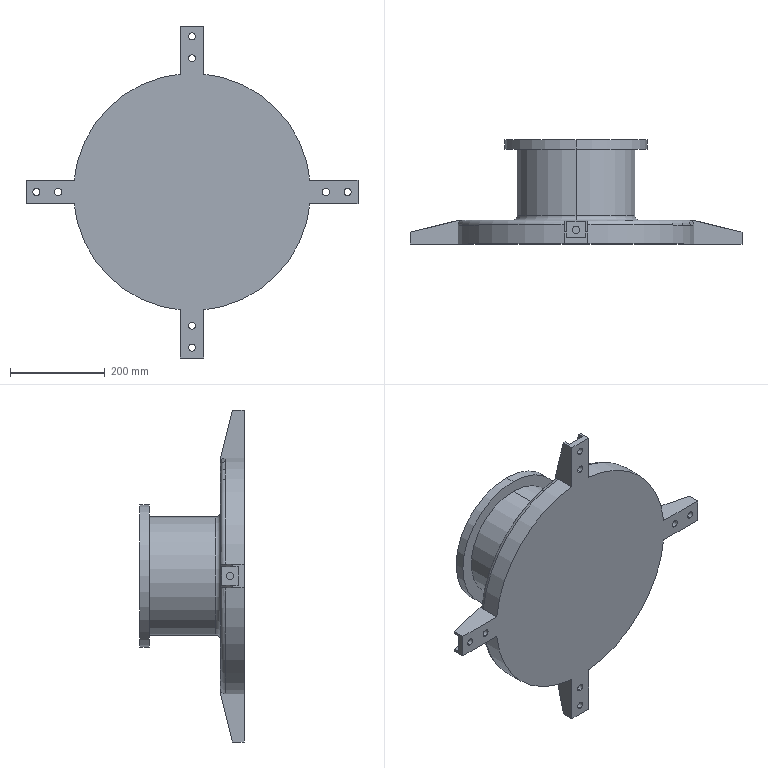Part | SolidWorks | features HoleWzd 6, ICE 5, BaseBody 1, Fillet 1, Revolution 1 | 1 solid | 81 faces | box 700 x 220 x 700 mm | volume 17727332 mm3 | plane 41 | cylinder 34 | torus 6 | commonest cylinder face diameters 15 x24 500 x4 125 x2 250 x2 300 x2